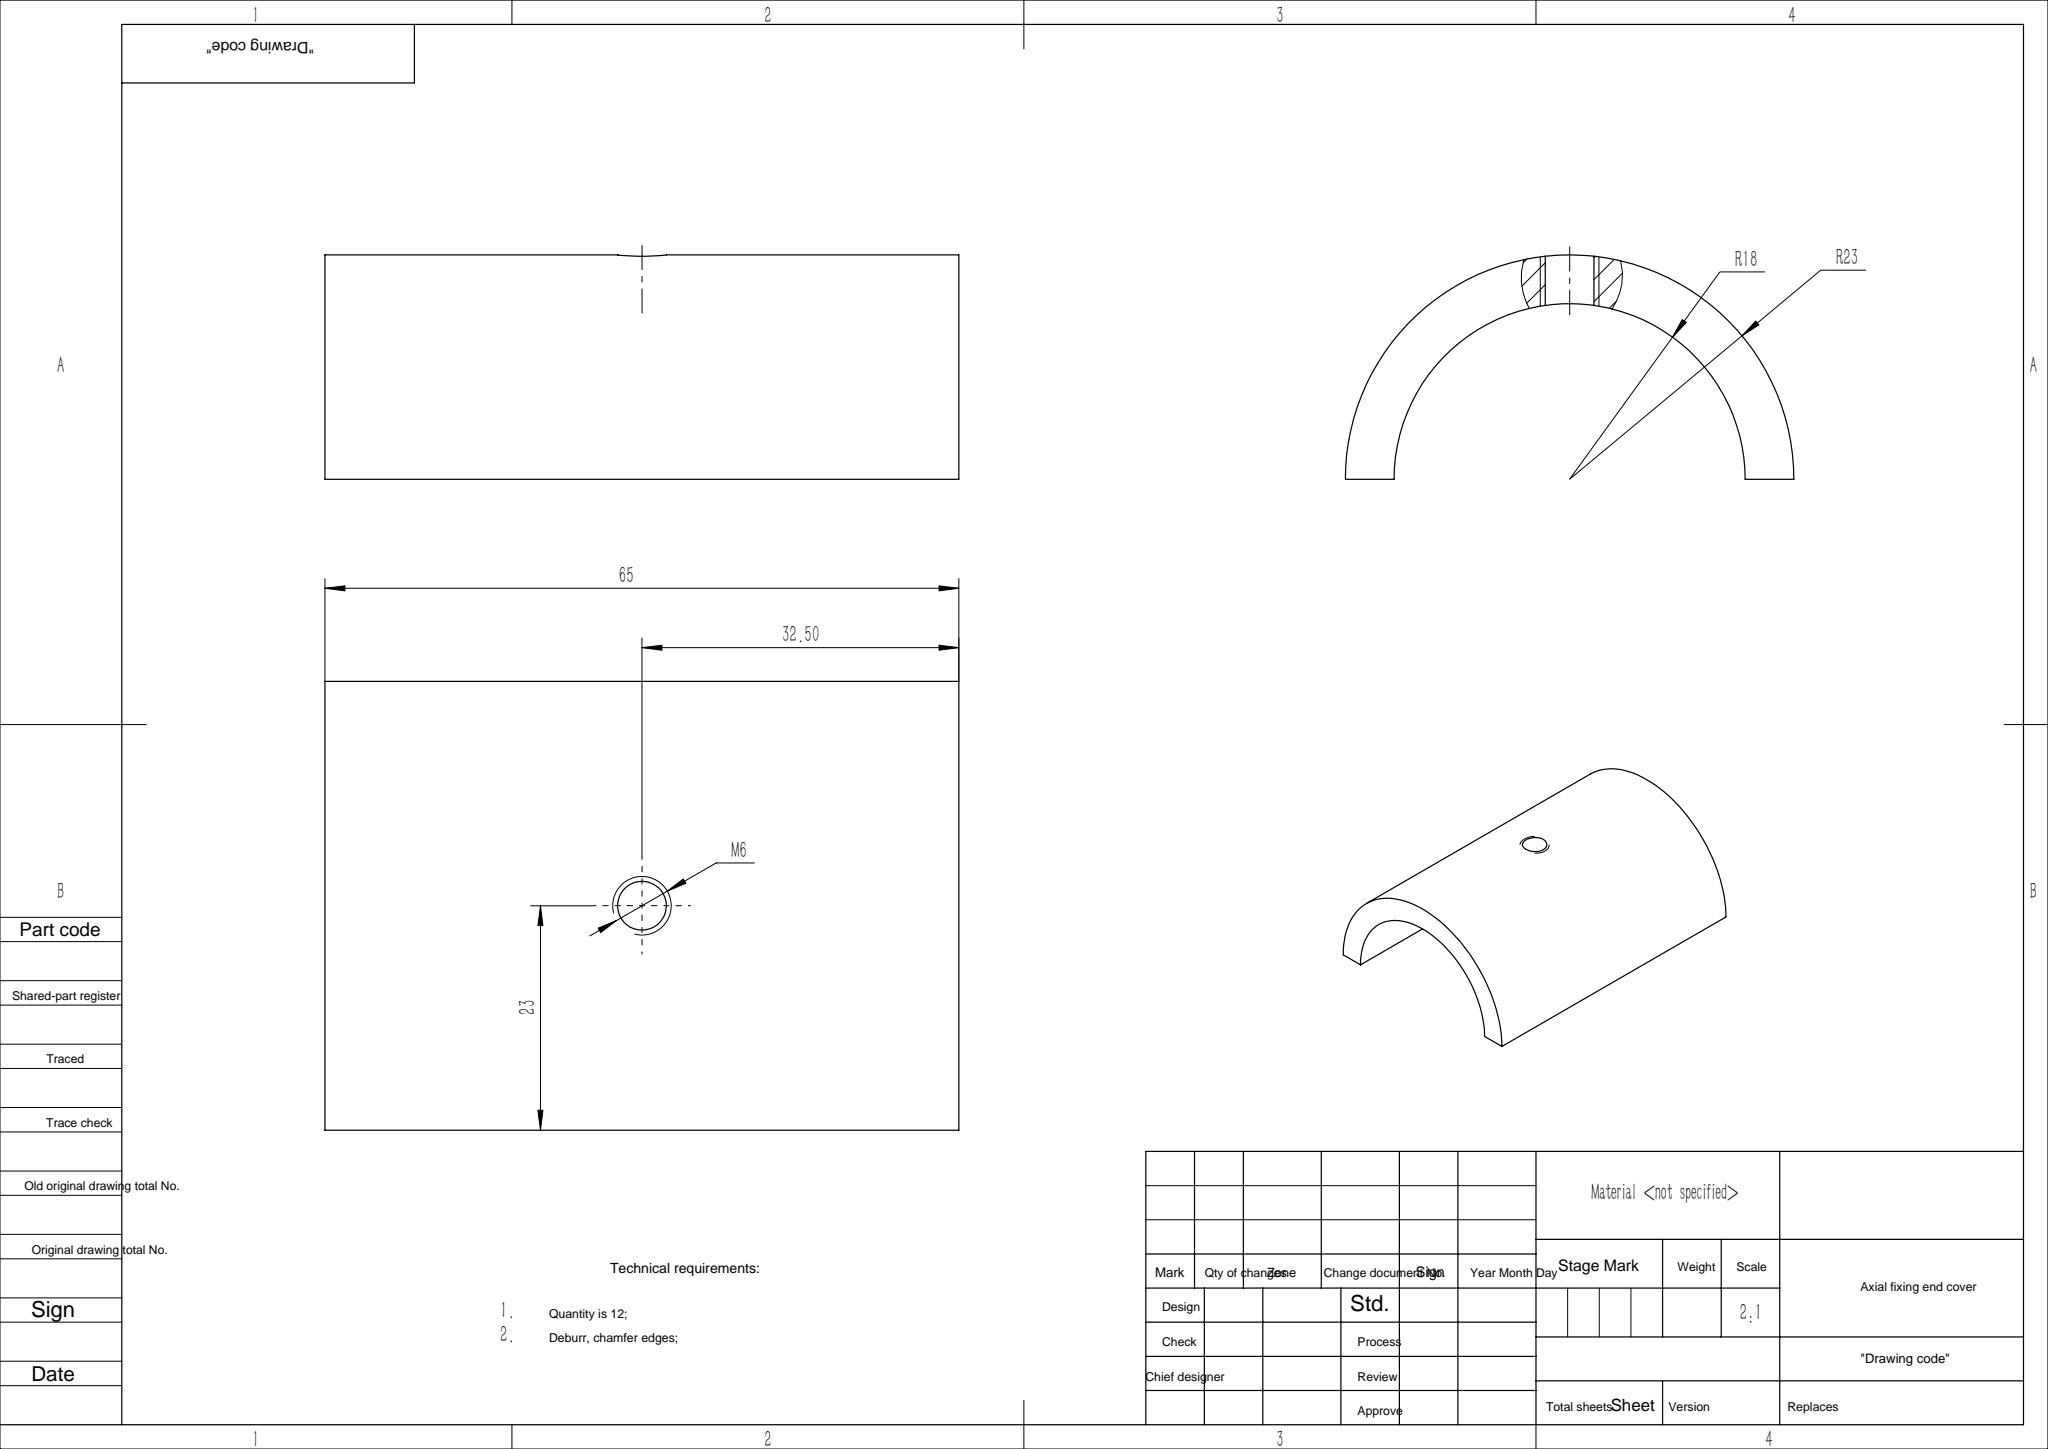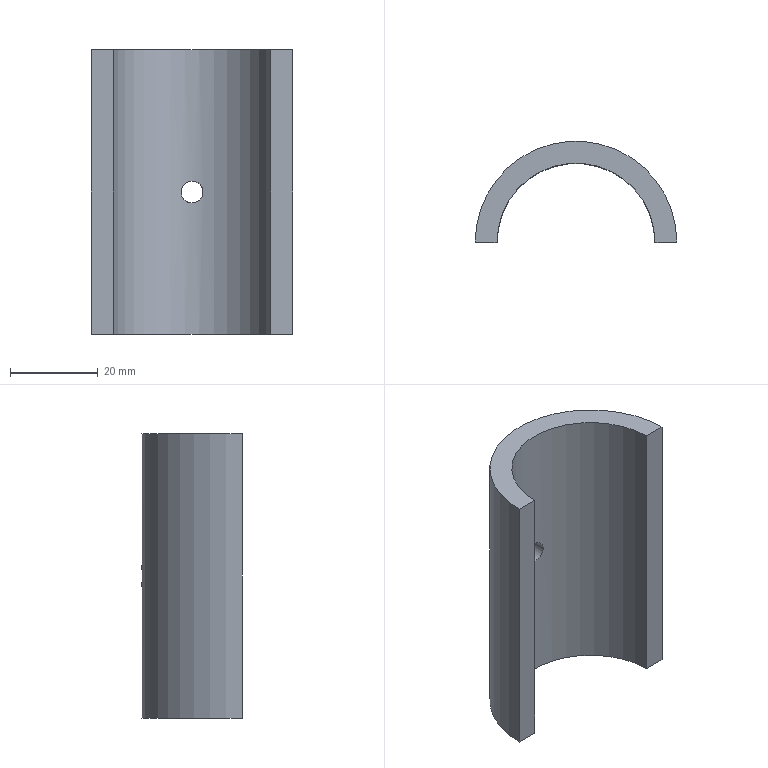Part | SolidWorks | features 3DProfileFeature 1, Extrusion 1, HoleWzd 1 | 1 solid | 8 faces | box 46 x 23 x 65 mm | volume 20833 mm3 | cylinder 4 | plane 4 | commonest cylinder face diameters 5 x2 36 x1 46 x1
STEP:
#1=CARTESIAN_POINT('',(0.,18.,-30.));
#2=VERTEX_POINT('',#1);
#3=CARTESIAN_POINT('',(0.,18.,-35.));
#4=VERTEX_POINT('',#3);
#5=CARTESIAN_POINT('',(0.,18.,-30.));
#6=CARTESIAN_POINT('',(-0.1654,18.,-30.));
#7=CARTESIAN_POINT('',(-0.328,17.998,-30.016));
#8=CARTESIAN_POINT('',(-0.6478,17.989,-30.08));
#9=CARTESIAN_POINT('',(-0.8067,17.983,-30.128));
#10=CARTESIAN_POINT('',(-1.109,17.966,-30.254));
#11=CARTESIAN_POINT('',(-1.253,17.957,-30.33));
#12=CARTESIAN_POINT('',(-1.525,17.936,-30.512));
#13=CARTESIAN_POINT('',(-1.653,17.924,-30.617));
#14=CARTESIAN_POINT('',(-1.883,17.902,-30.848));
#15=CARTESIAN_POINT('',(-1.987,17.89,-30.974));
#16=CARTESIAN_POINT('',(-2.169,17.869,-31.247));
#17=CARTESIAN_POINT('',(-2.247,17.859,-31.392));
#18=CARTESIAN_POINT('',(-2.372,17.843,-31.693));
#19=CARTESIAN_POINT('',(-2.42,17.837,-31.851));
#20=CARTESIAN_POINT('',(-2.484,17.828,-32.173));
#21=CARTESIAN_POINT('',(-2.5,17.826,-32.336));
#22=CARTESIAN_POINT('',(-2.5,17.826,-32.662));
#23=CARTESIAN_POINT('',(-2.484,17.828,-32.828));
#24=CARTESIAN_POINT('',(-2.42,17.837,-33.149));
#25=CARTESIAN_POINT('',(-2.373,17.843,-33.305));
#26=CARTESIAN_POINT('',(-2.247,17.859,-33.608));
#27=CARTESIAN_POINT('',(-2.169,17.869,-33.754));
#28=CARTESIAN_POINT('',(-1.988,17.89,-34.025));
#29=CARTESIAN_POINT('',(-1.884,17.901,-34.151));
#30=CARTESIAN_POINT('',(-1.651,17.924,-34.384));
#31=CARTESIAN_POINT('',(-1.525,17.936,-34.487));
#32=CARTESIAN_POINT('',(-1.255,17.957,-34.668));
#33=CARTESIAN_POINT('',(-1.108,17.966,-34.747));
#34=CARTESIAN_POINT('',(-0.8058,17.983,-34.872));
#35=CARTESIAN_POINT('',(-0.6499,17.989,-34.92));
#36=CARTESIAN_POINT('',(-0.3291,17.998,-34.984));
#37=CARTESIAN_POINT('',(-0.1633,18.,-35.));
#38=CARTESIAN_POINT('',(0.,18.,-35.));
#39=B_SPLINE_CURVE_WITH_KNOTS('',3,(#5,#6,#7,#8,#9,#10,#11,#12,#13,#14,#15,#16,#17,#18,#19,#20,#21,#22,#23,#24,#25,#26,#27,#28,#29,#30,#31,#32,#33,#34,#35,#36,#37,#38),.UNSPECIFIED.,.F.,.F.,(4,2,2,2,2,2,2,2,2,2,2,2,2,2,2,2,4),(0.,0.0004891,0.0009782,0.001467,0.001956,0.002445,0.002935,0.003424,0.003913,0.004402,0.004891,0.00538,0.005869,0.006358,0.006847,0.007336,0.007826),.UNSPECIFIED.);
#40=EDGE_CURVE('',#2,#4,#39,.T.);
#41=ORIENTED_EDGE('',*,*,#40,.T.);
#42=CARTESIAN_POINT('',(0.,23.,-35.));
#43=VERTEX_POINT('',#42);
#44=CARTESIAN_POINT('',(0.,23.,-35.));
#45=DIRECTION('',(0.,1.,0.));
#46=VECTOR('',#45,1000.);
#47=LINE('',#44,#46);
#48=EDGE_CURVE('',#4,#43,#47,.T.);
#49=ORIENTED_EDGE('',*,*,#48,.T.);
#50=CARTESIAN_POINT('',(0.,23.,-30.));
#51=VERTEX_POINT('',#50);
#52=CARTESIAN_POINT('',(0.,23.,-35.));
#53=CARTESIAN_POINT('',(-0.1632,23.,-35.));
#54=CARTESIAN_POINT('',(-0.3255,22.998,-34.984));
#55=CARTESIAN_POINT('',(-0.6481,22.991,-34.92));
#56=CARTESIAN_POINT('',(-0.8059,22.986,-34.872));
#57=CARTESIAN_POINT('',(-1.107,22.974,-34.748));
#58=CARTESIAN_POINT('',(-1.252,22.966,-34.67));
#59=CARTESIAN_POINT('',(-1.525,22.95,-34.487));
#60=CARTESIAN_POINT('',(-1.651,22.941,-34.384));
#61=CARTESIAN_POINT('',(-1.882,22.923,-34.154));
#62=CARTESIAN_POINT('',(-1.987,22.914,-34.025));
#63=CARTESIAN_POINT('',(-2.169,22.898,-33.754));
#64=CARTESIAN_POINT('',(-2.246,22.89,-33.61));
#65=CARTESIAN_POINT('',(-2.372,22.877,-33.308));
#66=CARTESIAN_POINT('',(-2.42,22.872,-33.149));
#67=CARTESIAN_POINT('',(-2.484,22.866,-32.83));
#68=CARTESIAN_POINT('',(-2.5,22.864,-32.667));
#69=CARTESIAN_POINT('',(-2.5,22.864,-32.337));
#70=CARTESIAN_POINT('',(-2.484,22.865,-32.174));
#71=CARTESIAN_POINT('',(-2.421,22.872,-31.854));
#72=CARTESIAN_POINT('',(-2.373,22.877,-31.696));
#73=CARTESIAN_POINT('',(-2.247,22.89,-31.393));
#74=CARTESIAN_POINT('',(-2.171,22.898,-31.249));
#75=CARTESIAN_POINT('',(-1.99,22.914,-30.977));
#76=CARTESIAN_POINT('',(-1.884,22.923,-30.849));
#77=CARTESIAN_POINT('',(-1.654,22.941,-30.618));
#78=CARTESIAN_POINT('',(-1.528,22.95,-30.515));
#79=CARTESIAN_POINT('',(-1.255,22.966,-30.332));
#80=CARTESIAN_POINT('',(-1.11,22.974,-30.254));
#81=CARTESIAN_POINT('',(-0.6589,22.993,-30.067));
#82=CARTESIAN_POINT('',(-0.3305,23.,-30.));
#83=CARTESIAN_POINT('',(0.,23.,-30.));
#84=B_SPLINE_CURVE_WITH_KNOTS('',3,(#52,#53,#54,#55,#56,#57,#58,#59,#60,#61,#62,#63,#64,#65,#66,#67,#68,#69,#70,#71,#72,#73,#74,#75,#76,#77,#78,#79,#80,#81,#82,#83),.UNSPECIFIED.,.F.,.F.,(4,2,2,2,2,2,2,2,2,2,2,2,2,2,2,4),(0.007822,0.008311,0.008799,0.009288,0.009777,0.01027,0.01075,0.01124,0.01173,0.01222,0.01271,0.0132,0.01369,0.01418,0.01466,0.01564),.UNSPECIFIED.);
#85=EDGE_CURVE('',#43,#51,#84,.T.);
#86=ORIENTED_EDGE('',*,*,#85,.T.);
#87=CARTESIAN_POINT('',(0.,23.,-30.));
#88=DIRECTION('',(0.,1.,0.));
#89=VECTOR('',#88,1000.);
#90=LINE('',#87,#89);
#91=EDGE_CURVE('',#2,#51,#90,.T.);
#92=ORIENTED_EDGE('',*,*,#91,.F.);
#93=EDGE_LOOP('',(#41,#49,#86,#92));
#94=FACE_OUTER_BOUND('',#93,.T.);
#95=CARTESIAN_POINT('',(0.,23.,-32.5));
#96=DIRECTION('',(0.,1.,0.));
#97=DIRECTION('',(0.,0.,1.));
#98=AXIS2_PLACEMENT_3D('',#95,#96,#97);
#99=CYLINDRICAL_SURFACE('',#98,2.5);
#100=ADVANCED_FACE('',(#94),#99,.F.);
#101=CARTESIAN_POINT('',(0.,23.,-30.));
#102=CARTESIAN_POINT('',(0.1653,23.,-30.));
#103=CARTESIAN_POINT('',(0.3278,22.998,-30.016));
#104=CARTESIAN_POINT('',(0.6475,22.991,-30.08));
#105=CARTESIAN_POINT('',(0.8064,22.986,-30.128));
#106=CARTESIAN_POINT('',(1.109,22.974,-30.254));
#107=CARTESIAN_POINT('',(1.253,22.966,-30.33));
#108=CARTESIAN_POINT('',(1.524,22.95,-30.512));
#109=CARTESIAN_POINT('',(1.653,22.941,-30.617));
#110=CARTESIAN_POINT('',(1.883,22.923,-30.848));
#111=CARTESIAN_POINT('',(1.987,22.914,-30.974));
#112=CARTESIAN_POINT('',(2.17,22.898,-31.247));
#113=CARTESIAN_POINT('',(2.247,22.89,-31.392));
#114=CARTESIAN_POINT('',(2.372,22.877,-31.693));
#115=CARTESIAN_POINT('',(2.42,22.872,-31.851));
#116=CARTESIAN_POINT('',(2.484,22.865,-32.174));
#117=CARTESIAN_POINT('',(2.5,22.864,-32.336));
#118=CARTESIAN_POINT('',(2.5,22.864,-32.662));
#119=CARTESIAN_POINT('',(2.484,22.866,-32.828));
#120=CARTESIAN_POINT('',(2.42,22.872,-33.149));
#121=CARTESIAN_POINT('',(2.373,22.877,-33.305));
#122=CARTESIAN_POINT('',(2.247,22.89,-33.608));
#123=CARTESIAN_POINT('',(2.169,22.898,-33.754));
#124=CARTESIAN_POINT('',(1.988,22.914,-34.025));
#125=CARTESIAN_POINT('',(1.885,22.923,-34.151));
#126=CARTESIAN_POINT('',(1.651,22.941,-34.384));
#127=CARTESIAN_POINT('',(1.525,22.95,-34.488));
#128=CARTESIAN_POINT('',(1.254,22.966,-34.669));
#129=CARTESIAN_POINT('',(1.108,22.974,-34.747));
#130=CARTESIAN_POINT('',(0.8055,22.986,-34.872));
#131=CARTESIAN_POINT('',(0.6496,22.991,-34.92));
#132=CARTESIAN_POINT('',(0.329,22.998,-34.984));
#133=CARTESIAN_POINT('',(0.1632,23.,-35.));
#134=CARTESIAN_POINT('',(0.,23.,-35.));
#135=B_SPLINE_CURVE_WITH_KNOTS('',3,(#101,#102,#103,#104,#105,#106,#107,#108,#109,#110,#111,#112,#113,#114,#115,#116,#117,#118,#119,#120,#121,#122,#123,#124,#125,#126,#127,#128,#129,#130,#131,#132,#133,#134),.UNSPECIFIED.,.F.,.F.,(4,2,2,2,2,2,2,2,2,2,2,2,2,2,2,2,4),(0.,0.0004889,0.0009777,0.001467,0.001955,0.002444,0.002933,0.003422,0.003911,0.0044,0.004889,0.005378,0.005866,0.006355,0.006844,0.007333,0.007822),.UNSPECIFIED.);
#136=EDGE_CURVE('',#51,#43,#135,.T.);
#137=ORIENTED_EDGE('',*,*,#136,.F.);
#138=ORIENTED_EDGE('',*,*,#85,.F.);
#139=EDGE_LOOP('',(#137,#138));
#140=FACE_BOUND('',#139,.T.);
#141=CARTESIAN_POINT('',(23.,0.,0.));
#142=VERTEX_POINT('',#141);
#143=CARTESIAN_POINT('',(-23.,0.,0.));
#144=VERTEX_POINT('',#143);
#145=CARTESIAN_POINT('',(0.,0.,0.));
#146=DIRECTION('',(0.,0.,1.));
#147=DIRECTION('',(1.,0.,0.));
#148=AXIS2_PLACEMENT_3D('',#145,#146,#147);
#149=CIRCLE('',#148,23.);
#150=EDGE_CURVE('',#142,#144,#149,.T.);
#151=ORIENTED_EDGE('',*,*,#150,.F.);
#152=CARTESIAN_POINT('',(23.,0.,-65.));
#153=VERTEX_POINT('',#152);
#154=CARTESIAN_POINT('',(23.,0.,-65.));
#155=DIRECTION('',(0.,0.,1.));
#156=VECTOR('',#155,1000.);
#157=LINE('',#154,#156);
#158=EDGE_CURVE('',#153,#142,#157,.T.);
#159=ORIENTED_EDGE('',*,*,#158,.F.);
#160=CARTESIAN_POINT('',(-23.,0.,-65.));
#161=VERTEX_POINT('',#160);
#162=CARTESIAN_POINT('',(0.,0.,-65.));
#163=DIRECTION('',(0.,0.,1.));
#164=DIRECTION('',(1.,0.,0.));
#165=AXIS2_PLACEMENT_3D('',#162,#163,#164);
#166=CIRCLE('',#165,23.);
#167=EDGE_CURVE('',#153,#161,#166,.T.);
#168=ORIENTED_EDGE('',*,*,#167,.T.);
#169=CARTESIAN_POINT('',(-23.,0.,-65.));
#170=DIRECTION('',(0.,0.,1.));
#171=VECTOR('',#170,1000.);
#172=LINE('',#169,#171);
#173=EDGE_CURVE('',#161,#144,#172,.T.);
#174=ORIENTED_EDGE('',*,*,#173,.T.);
#175=EDGE_LOOP('',(#151,#159,#168,#174));
#176=FACE_OUTER_BOUND('',#175,.T.);
#177=CARTESIAN_POINT('',(0.,0.,-65.));
#178=DIRECTION('',(0.,0.,1.));
#179=DIRECTION('',(1.,0.,0.));
#180=AXIS2_PLACEMENT_3D('',#177,#178,#179);
#181=CYLINDRICAL_SURFACE('',#180,23.);
#182=ADVANCED_FACE('',(#140,#176),#181,.T.);
#183=CARTESIAN_POINT('',(18.,0.,0.));
#184=VERTEX_POINT('',#183);
#185=CARTESIAN_POINT('',(18.,0.,0.));
#186=DIRECTION('',(1.,0.,0.));
#187=VECTOR('',#186,1000.);
#188=LINE('',#185,#187);
#189=EDGE_CURVE('',#184,#142,#188,.T.);
#190=ORIENTED_EDGE('',*,*,#189,.F.);
#191=CARTESIAN_POINT('',(18.,0.,-65.));
#192=VERTEX_POINT('',#191);
#193=CARTESIAN_POINT('',(18.,0.,-65.));
#194=DIRECTION('',(0.,0.,1.));
#195=VECTOR('',#194,1000.);
#196=LINE('',#193,#195);
#197=EDGE_CURVE('',#192,#184,#196,.T.);
#198=ORIENTED_EDGE('',*,*,#197,.F.);
#199=CARTESIAN_POINT('',(18.,0.,-65.));
#200=DIRECTION('',(1.,0.,0.));
#201=VECTOR('',#200,1000.);
#202=LINE('',#199,#201);
#203=EDGE_CURVE('',#192,#153,#202,.T.);
#204=ORIENTED_EDGE('',*,*,#203,.T.);
#205=ORIENTED_EDGE('',*,*,#158,.T.);
#206=EDGE_LOOP('',(#190,#198,#204,#205));
#207=FACE_OUTER_BOUND('',#206,.T.);
#208=CARTESIAN_POINT('',(18.,0.,-65.));
#209=DIRECTION('',(0.,-1.,0.));
#210=DIRECTION('',(0.,0.,-1.));
#211=AXIS2_PLACEMENT_3D('',#208,#209,#210);
#212=PLANE('',#211);
#213=ADVANCED_FACE('',(#207),#212,.T.);
#214=ORIENTED_EDGE('',*,*,#40,.F.);
#215=CARTESIAN_POINT('',(0.,18.,-35.));
#216=CARTESIAN_POINT('',(0.1632,18.,-35.));
#217=CARTESIAN_POINT('',(0.3256,17.998,-34.984));
#218=CARTESIAN_POINT('',(0.6486,17.989,-34.92));
#219=CARTESIAN_POINT('',(0.8062,17.983,-34.872));
#220=CARTESIAN_POINT('',(1.107,17.967,-34.747));
#221=CARTESIAN_POINT('',(1.253,17.957,-34.67));
#222=CARTESIAN_POINT('',(1.526,17.936,-34.487));
#223=CARTESIAN_POINT('',(1.651,17.924,-34.384));
#224=CARTESIAN_POINT('',(1.882,17.902,-34.154));
#225=CARTESIAN_POINT('',(1.987,17.89,-34.025));
#226=CARTESIAN_POINT('',(2.169,17.869,-33.754));
#227=CARTESIAN_POINT('',(2.246,17.859,-33.611));
#228=CARTESIAN_POINT('',(2.371,17.843,-33.308));
#229=CARTESIAN_POINT('',(2.42,17.837,-33.149));
#230=CARTESIAN_POINT('',(2.484,17.828,-32.83));
#231=CARTESIAN_POINT('',(2.5,17.826,-32.667));
#232=CARTESIAN_POINT('',(2.5,17.826,-32.336));
#233=CARTESIAN_POINT('',(2.484,17.828,-32.174));
#234=CARTESIAN_POINT('',(2.421,17.837,-31.854));
#235=CARTESIAN_POINT('',(2.373,17.843,-31.695));
#236=CARTESIAN_POINT('',(2.247,17.859,-31.392));
#237=CARTESIAN_POINT('',(2.171,17.869,-31.249));
#238=CARTESIAN_POINT('',(1.989,17.89,-30.977));
#239=CARTESIAN_POINT('',(1.884,17.902,-30.849));
#240=CARTESIAN_POINT('',(1.539,17.936,-30.503));
#241=CARTESIAN_POINT('',(1.26,17.958,-30.317));
#242=CARTESIAN_POINT('',(0.6593,17.99,-30.067));
#243=CARTESIAN_POINT('',(0.3307,18.,-30.));
#244=CARTESIAN_POINT('',(0.,18.,-30.));
#245=B_SPLINE_CURVE_WITH_KNOTS('',3,(#215,#216,#217,#218,#219,#220,#221,#222,#223,#224,#225,#226,#227,#228,#229,#230,#231,#232,#233,#234,#235,#236,#237,#238,#239,#240,#241,#242,#243,#244),.UNSPECIFIED.,.F.,.F.,(4,2,2,2,2,2,2,2,2,2,2,2,2,2,4),(0.007826,0.008315,0.008804,0.009293,0.009782,0.01027,0.01076,0.01125,0.01174,0.01223,0.01272,0.0132,0.01369,0.01467,0.01565),.UNSPECIFIED.);
#246=EDGE_CURVE('',#4,#2,#245,.T.);
#247=ORIENTED_EDGE('',*,*,#246,.F.);
#248=EDGE_LOOP('',(#214,#247));
#249=FACE_BOUND('',#248,.T.);
#250=CARTESIAN_POINT('',(-18.,0.,0.));
#251=VERTEX_POINT('',#250);
#252=CARTESIAN_POINT('',(0.,0.,0.));
#253=DIRECTION('',(0.,0.,-1.));
#254=DIRECTION('',(1.,0.,0.));
#255=AXIS2_PLACEMENT_3D('',#252,#253,#254);
#256=CIRCLE('',#255,18.);
#257=EDGE_CURVE('',#251,#184,#256,.T.);
#258=ORIENTED_EDGE('',*,*,#257,.F.);
#259=CARTESIAN_POINT('',(-18.,0.,-65.));
#260=VERTEX_POINT('',#259);
#261=CARTESIAN_POINT('',(-18.,0.,-65.));
#262=DIRECTION('',(0.,0.,1.));
#263=VECTOR('',#262,1000.);
#264=LINE('',#261,#263);
#265=EDGE_CURVE('',#260,#251,#264,.T.);
#266=ORIENTED_EDGE('',*,*,#265,.F.);
#267=CARTESIAN_POINT('',(0.,0.,-65.));
#268=DIRECTION('',(0.,0.,-1.));
#269=DIRECTION('',(1.,0.,0.));
#270=AXIS2_PLACEMENT_3D('',#267,#268,#269);
#271=CIRCLE('',#270,18.);
#272=EDGE_CURVE('',#260,#192,#271,.T.);
#273=ORIENTED_EDGE('',*,*,#272,.T.);
#274=ORIENTED_EDGE('',*,*,#197,.T.);
#275=EDGE_LOOP('',(#258,#266,#273,#274));
#276=FACE_OUTER_BOUND('',#275,.T.);
#277=CARTESIAN_POINT('',(0.,0.,-65.));
#278=DIRECTION('',(0.,0.,1.));
#279=DIRECTION('',(1.,0.,0.));
#280=AXIS2_PLACEMENT_3D('',#277,#278,#279);
#281=CYLINDRICAL_SURFACE('',#280,18.);
#282=ADVANCED_FACE('',(#249,#276),#281,.F.);
#283=CARTESIAN_POINT('',(-23.,0.,0.));
#284=DIRECTION('',(1.,0.,0.));
#285=VECTOR('',#284,1000.);
#286=LINE('',#283,#285);
#287=EDGE_CURVE('',#144,#251,#286,.T.);
#288=ORIENTED_EDGE('',*,*,#287,.F.);
#289=ORIENTED_EDGE('',*,*,#173,.F.);
#290=CARTESIAN_POINT('',(-23.,0.,-65.));
#291=DIRECTION('',(1.,0.,0.));
#292=VECTOR('',#291,1000.);
#293=LINE('',#290,#292);
#294=EDGE_CURVE('',#161,#260,#293,.T.);
#295=ORIENTED_EDGE('',*,*,#294,.T.);
#296=ORIENTED_EDGE('',*,*,#265,.T.);
#297=EDGE_LOOP('',(#288,#289,#295,#296));
#298=FACE_OUTER_BOUND('',#297,.T.);
#299=CARTESIAN_POINT('',(-23.,0.,-65.));
#300=DIRECTION('',(0.,-1.,0.));
#301=DIRECTION('',(0.,0.,-1.));
#302=AXIS2_PLACEMENT_3D('',#299,#300,#301);
#303=PLANE('',#302);
#304=ADVANCED_FACE('',(#298),#303,.T.);
#305=ORIENTED_EDGE('',*,*,#167,.F.);
#306=ORIENTED_EDGE('',*,*,#203,.F.);
#307=ORIENTED_EDGE('',*,*,#272,.F.);
#308=ORIENTED_EDGE('',*,*,#294,.F.);
#309=EDGE_LOOP('',(#305,#306,#307,#308));
#310=FACE_OUTER_BOUND('',#309,.T.);
#311=CARTESIAN_POINT('',(0.,0.,-65.));
#312=DIRECTION('',(0.,0.,1.));
#313=DIRECTION('',(1.,0.,0.));
#314=AXIS2_PLACEMENT_3D('',#311,#312,#313);
#315=PLANE('',#314);
#316=ADVANCED_FACE('',(#310),#315,.F.);
#317=ORIENTED_EDGE('',*,*,#150,.T.);
#318=ORIENTED_EDGE('',*,*,#287,.T.);
#319=ORIENTED_EDGE('',*,*,#257,.T.);
#320=ORIENTED_EDGE('',*,*,#189,.T.);
#321=EDGE_LOOP('',(#317,#318,#319,#320));
#322=FACE_OUTER_BOUND('',#321,.T.);
#323=CARTESIAN_POINT('',(0.,0.,0.));
#324=DIRECTION('',(0.,0.,1.));
#325=DIRECTION('',(1.,0.,0.));
#326=AXIS2_PLACEMENT_3D('',#323,#324,#325);
#327=PLANE('',#326);
#328=ADVANCED_FACE('',(#322),#327,.T.);
#329=ORIENTED_EDGE('',*,*,#48,.F.);
#330=ORIENTED_EDGE('',*,*,#246,.T.);
#331=ORIENTED_EDGE('',*,*,#91,.T.);
#332=ORIENTED_EDGE('',*,*,#136,.T.);
#333=EDGE_LOOP('',(#329,#330,#331,#332));
#334=FACE_OUTER_BOUND('',#333,.T.);
#335=CARTESIAN_POINT('',(0.,23.,-32.5));
#336=DIRECTION('',(0.,1.,0.));
#337=DIRECTION('',(0.,0.,1.));
#338=AXIS2_PLACEMENT_3D('',#335,#336,#337);
#339=CYLINDRICAL_SURFACE('',#338,2.5);
#340=ADVANCED_FACE('',(#334),#339,.F.);
#341=CLOSED_SHELL('',(#100,#182,#213,#282,#304,#316,#328,#340));
#342=MANIFOLD_SOLID_BREP('',#341);
#343=CARTESIAN_POINT('',(0.,0.,0.));
#344=DIRECTION('',(0.,0.,1.));
#345=DIRECTION('',(1.,0.,0.));
#346=AXIS2_PLACEMENT_3D('',#343,#344,#345);
#347=(LENGTH_UNIT()NAMED_UNIT(*)SI_UNIT(.MILLI.,.METRE.));
#348=UNCERTAINTY_MEASURE_WITH_UNIT(LENGTH_MEASURE(0.00001),#347,'','');
#349=(NAMED_UNIT(*)PLANE_ANGLE_UNIT()SI_UNIT($,.RADIAN.));
#350=(NAMED_UNIT(*)SI_UNIT($,.STERADIAN.)SOLID_ANGLE_UNIT());
#351=(GEOMETRIC_REPRESENTATION_CONTEXT(3)GLOBAL_UNCERTAINTY_ASSIGNED_CONTEXT((#348))GLOBAL_UNIT_ASSIGNED_CONTEXT((#347,#349,#350))REPRESENTATION_CONTEXT('',''));
#352=ADVANCED_BREP_SHAPE_REPRESENTATION('',(#342,#346),#351);